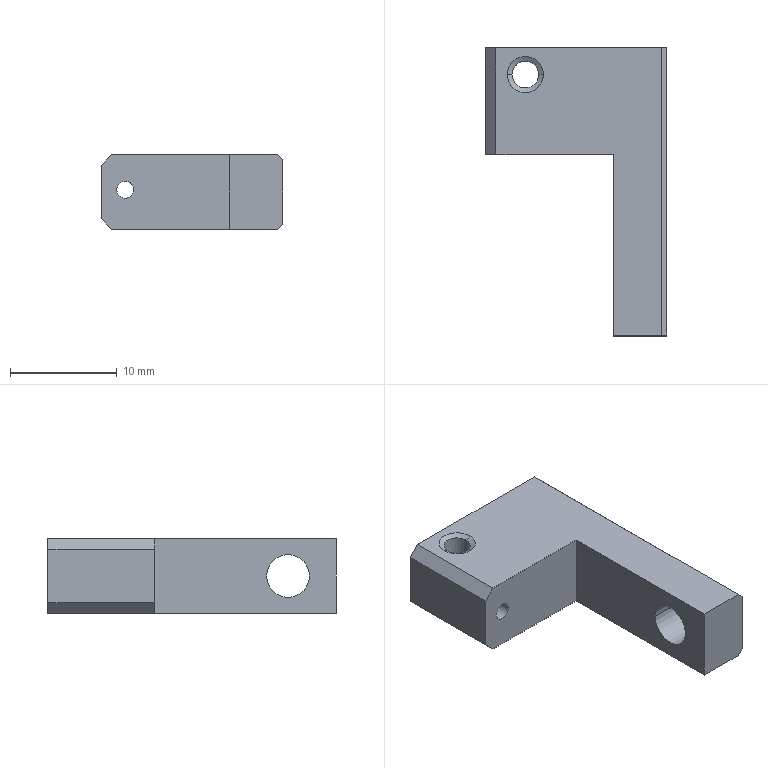Part | NX | 1 solid | 20 faces | box 17 x 27 x 7 mm | volume 1651 mm3 | plane 12 | cylinder 6 | cone 2 | commonest cylinder face diameters 1.6 x2 2.5 x2 4 x2
STEP:
#1=CARTESIAN_POINT('',(1.,17.,0.));
#2=VERTEX_POINT('',#1);
#3=CARTESIAN_POINT('',(12.,17.,0.));
#4=VERTEX_POINT('',#3);
#5=CARTESIAN_POINT('',(0.,17.,0.));
#6=DIRECTION('',(1.,0.,0.));
#7=VECTOR('',#6,1000.);
#8=LINE('',#5,#7);
#9=EDGE_CURVE('',#2,#4,#8,.T.);
#10=ORIENTED_EDGE('',*,*,#9,.T.);
#11=CARTESIAN_POINT('',(12.,17.,7.));
#12=VERTEX_POINT('',#11);
#13=CARTESIAN_POINT('',(12.,17.,0.));
#14=DIRECTION('',(0.,0.,1.));
#15=VECTOR('',#14,1000.);
#16=LINE('',#13,#15);
#17=EDGE_CURVE('',#4,#12,#16,.T.);
#18=ORIENTED_EDGE('',*,*,#17,.T.);
#19=CARTESIAN_POINT('',(1.,17.,7.));
#20=VERTEX_POINT('',#19);
#21=CARTESIAN_POINT('',(0.,17.,7.));
#22=DIRECTION('',(1.,0.,0.));
#23=VECTOR('',#22,1000.);
#24=LINE('',#21,#23);
#25=EDGE_CURVE('',#20,#12,#24,.T.);
#26=ORIENTED_EDGE('',*,*,#25,.F.);
#27=CARTESIAN_POINT('',(0.,17.,6.));
#28=VERTEX_POINT('',#27);
#29=CARTESIAN_POINT('',(-6.,17.,0.));
#30=DIRECTION('',(0.7071,0.,0.7071));
#31=VECTOR('',#30,1000.);
#32=LINE('',#29,#31);
#33=EDGE_CURVE('',#28,#20,#32,.T.);
#34=ORIENTED_EDGE('',*,*,#33,.F.);
#35=CARTESIAN_POINT('',(0.,17.,1.));
#36=VERTEX_POINT('',#35);
#37=CARTESIAN_POINT('',(0.,17.,0.));
#38=DIRECTION('',(0.,0.,-1.));
#39=VECTOR('',#38,1000.);
#40=LINE('',#37,#39);
#41=EDGE_CURVE('',#28,#36,#40,.T.);
#42=ORIENTED_EDGE('',*,*,#41,.T.);
#43=CARTESIAN_POINT('',(1.,17.,0.));
#44=DIRECTION('',(0.7071,0.,-0.7071));
#45=VECTOR('',#44,1000.);
#46=LINE('',#43,#45);
#47=EDGE_CURVE('',#36,#2,#46,.T.);
#48=ORIENTED_EDGE('',*,*,#47,.T.);
#49=EDGE_LOOP('',(#10,#18,#26,#34,#42,#48));
#50=FACE_BOUND('',#49,.T.);
#51=CARTESIAN_POINT('',(3.05,17.,3.7));
#52=VERTEX_POINT('',#51);
#53=CARTESIAN_POINT('',(1.45,17.,3.7));
#54=VERTEX_POINT('',#53);
#55=CARTESIAN_POINT('',(2.25,17.,3.7));
#56=DIRECTION('',(0.,-1.,0.));
#57=DIRECTION('',(1.,0.,0.));
#58=AXIS2_PLACEMENT_3D('',#55,#56,#57);
#59=CIRCLE('',#58,0.8);
#60=EDGE_CURVE('',#52,#54,#59,.T.);
#61=ORIENTED_EDGE('',*,*,#60,.F.);
#62=CARTESIAN_POINT('',(2.25,17.,3.7));
#63=DIRECTION('',(0.,-1.,0.));
#64=DIRECTION('',(1.,0.,0.));
#65=AXIS2_PLACEMENT_3D('',#62,#63,#64);
#66=CIRCLE('',#65,0.8);
#67=EDGE_CURVE('',#54,#52,#66,.T.);
#68=ORIENTED_EDGE('',*,*,#67,.F.);
#69=EDGE_LOOP('',(#61,#68));
#70=FACE_BOUND('',#69,.T.);
#71=CARTESIAN_POINT('',(12.,17.,7.));
#72=DIRECTION('',(0.,1.,0.));
#73=DIRECTION('',(1.,0.,0.));
#74=AXIS2_PLACEMENT_3D('',#71,#72,#73);
#75=PLANE('',#74);
#76=ADVANCED_FACE('',(#50,#70),#75,.F.);
#77=CARTESIAN_POINT('',(17.,27.,0.5));
#78=VERTEX_POINT('',#77);
#79=CARTESIAN_POINT('',(17.,0.,0.5));
#80=VERTEX_POINT('',#79);
#81=CARTESIAN_POINT('',(17.,27.,0.5));
#82=DIRECTION('',(0.,-1.,0.));
#83=VECTOR('',#82,1000.);
#84=LINE('',#81,#83);
#85=EDGE_CURVE('',#78,#80,#84,.T.);
#86=ORIENTED_EDGE('',*,*,#85,.F.);
#87=CARTESIAN_POINT('',(17.,27.,6.5));
#88=VERTEX_POINT('',#87);
#89=CARTESIAN_POINT('',(17.,27.,0.));
#90=DIRECTION('',(0.,0.,1.));
#91=VECTOR('',#90,1000.);
#92=LINE('',#89,#91);
#93=EDGE_CURVE('',#78,#88,#92,.T.);
#94=ORIENTED_EDGE('',*,*,#93,.T.);
#95=CARTESIAN_POINT('',(17.,0.,6.5));
#96=VERTEX_POINT('',#95);
#97=CARTESIAN_POINT('',(17.,27.,6.5));
#98=DIRECTION('',(0.,-1.,0.));
#99=VECTOR('',#98,1000.);
#100=LINE('',#97,#99);
#101=EDGE_CURVE('',#88,#96,#100,.T.);
#102=ORIENTED_EDGE('',*,*,#101,.T.);
#103=CARTESIAN_POINT('',(17.,0.,6.5));
#104=DIRECTION('',(0.,0.,-1.));
#105=VECTOR('',#104,1000.);
#106=LINE('',#103,#105);
#107=EDGE_CURVE('',#96,#80,#106,.T.);
#108=ORIENTED_EDGE('',*,*,#107,.T.);
#109=EDGE_LOOP('',(#86,#94,#102,#108));
#110=FACE_BOUND('',#109,.T.);
#111=CARTESIAN_POINT('',(17.,2.5,3.5));
#112=VERTEX_POINT('',#111);
#113=CARTESIAN_POINT('',(17.,6.5,3.5));
#114=VERTEX_POINT('',#113);
#115=CARTESIAN_POINT('',(17.,4.5,3.5));
#116=DIRECTION('',(1.,0.,0.));
#117=DIRECTION('',(0.,-1.,0.));
#118=AXIS2_PLACEMENT_3D('',#115,#116,#117);
#119=CIRCLE('',#118,2.);
#120=EDGE_CURVE('',#112,#114,#119,.T.);
#121=ORIENTED_EDGE('',*,*,#120,.F.);
#122=CARTESIAN_POINT('',(17.,4.5,3.5));
#123=DIRECTION('',(1.,0.,0.));
#124=DIRECTION('',(0.,-1.,0.));
#125=AXIS2_PLACEMENT_3D('',#122,#123,#124);
#126=CIRCLE('',#125,2.);
#127=EDGE_CURVE('',#114,#112,#126,.T.);
#128=ORIENTED_EDGE('',*,*,#127,.F.);
#129=EDGE_LOOP('',(#121,#128));
#130=FACE_BOUND('',#129,.T.);
#131=CARTESIAN_POINT('',(17.,0.,0.));
#132=DIRECTION('',(1.,0.,0.));
#133=DIRECTION('',(0.,1.,0.));
#134=AXIS2_PLACEMENT_3D('',#131,#132,#133);
#135=PLANE('',#134);
#136=ADVANCED_FACE('',(#110,#130),#135,.T.);
#137=CARTESIAN_POINT('',(12.,0.,7.));
#138=VERTEX_POINT('',#137);
#139=CARTESIAN_POINT('',(12.,0.,7.));
#140=DIRECTION('',(0.,-1.,0.));
#141=VECTOR('',#140,1000.);
#142=LINE('',#139,#141);
#143=EDGE_CURVE('',#12,#138,#142,.T.);
#144=ORIENTED_EDGE('',*,*,#143,.T.);
#145=CARTESIAN_POINT('',(16.5,0.,7.));
#146=VERTEX_POINT('',#145);
#147=CARTESIAN_POINT('',(0.,0.,7.));
#148=DIRECTION('',(-1.,0.,0.));
#149=VECTOR('',#148,1000.);
#150=LINE('',#147,#149);
#151=EDGE_CURVE('',#146,#138,#150,.T.);
#152=ORIENTED_EDGE('',*,*,#151,.F.);
#153=CARTESIAN_POINT('',(16.5,27.,7.));
#154=VERTEX_POINT('',#153);
#155=CARTESIAN_POINT('',(16.5,0.,7.));
#156=DIRECTION('',(0.,1.,0.));
#157=VECTOR('',#156,1000.);
#158=LINE('',#155,#157);
#159=EDGE_CURVE('',#146,#154,#158,.T.);
#160=ORIENTED_EDGE('',*,*,#159,.T.);
#161=CARTESIAN_POINT('',(1.,27.,7.));
#162=VERTEX_POINT('',#161);
#163=CARTESIAN_POINT('',(0.,27.,7.));
#164=DIRECTION('',(1.,0.,0.));
#165=VECTOR('',#164,1000.);
#166=LINE('',#163,#165);
#167=EDGE_CURVE('',#162,#154,#166,.T.);
#168=ORIENTED_EDGE('',*,*,#167,.F.);
#169=CARTESIAN_POINT('',(1.,0.,7.));
#170=DIRECTION('',(0.,-1.,0.));
#171=VECTOR('',#170,1000.);
#172=LINE('',#169,#171);
#173=EDGE_CURVE('',#162,#20,#172,.T.);
#174=ORIENTED_EDGE('',*,*,#173,.T.);
#175=ORIENTED_EDGE('',*,*,#25,.T.);
#176=EDGE_LOOP('',(#144,#152,#160,#168,#174,#175));
#177=FACE_BOUND('',#176,.T.);
#178=CARTESIAN_POINT('',(5.45,24.5,7.));
#179=VERTEX_POINT('',#178);
#180=CARTESIAN_POINT('',(2.05,24.5,7.));
#181=VERTEX_POINT('',#180);
#182=CARTESIAN_POINT('',(3.75,24.5,7.));
#183=DIRECTION('',(0.,0.,1.));
#184=DIRECTION('',(1.,0.,0.));
#185=AXIS2_PLACEMENT_3D('',#182,#183,#184);
#186=CIRCLE('',#185,1.7);
#187=EDGE_CURVE('',#179,#181,#186,.T.);
#188=ORIENTED_EDGE('',*,*,#187,.F.);
#189=CARTESIAN_POINT('',(3.75,24.5,7.));
#190=DIRECTION('',(0.,0.,1.));
#191=DIRECTION('',(1.,0.,0.));
#192=AXIS2_PLACEMENT_3D('',#189,#190,#191);
#193=CIRCLE('',#192,1.7);
#194=EDGE_CURVE('',#181,#179,#193,.T.);
#195=ORIENTED_EDGE('',*,*,#194,.F.);
#196=EDGE_LOOP('',(#188,#195));
#197=FACE_BOUND('',#196,.T.);
#198=CARTESIAN_POINT('',(0.,0.,7.));
#199=DIRECTION('',(0.,0.,1.));
#200=DIRECTION('',(1.,0.,0.));
#201=AXIS2_PLACEMENT_3D('',#198,#199,#200);
#202=PLANE('',#201);
#203=ADVANCED_FACE('',(#177,#197),#202,.T.);
#204=CARTESIAN_POINT('',(1.,27.,0.));
#205=VERTEX_POINT('',#204);
#206=CARTESIAN_POINT('',(1.,0.,0.));
#207=DIRECTION('',(0.,1.,0.));
#208=VECTOR('',#207,1000.);
#209=LINE('',#206,#208);
#210=EDGE_CURVE('',#2,#205,#209,.T.);
#211=ORIENTED_EDGE('',*,*,#210,.F.);
#212=ORIENTED_EDGE('',*,*,#47,.F.);
#213=CARTESIAN_POINT('',(0.,27.,1.));
#214=VERTEX_POINT('',#213);
#215=CARTESIAN_POINT('',(0.,17.,1.));
#216=DIRECTION('',(0.,1.,0.));
#217=VECTOR('',#216,1000.);
#218=LINE('',#215,#217);
#219=EDGE_CURVE('',#36,#214,#218,.T.);
#220=ORIENTED_EDGE('',*,*,#219,.T.);
#221=CARTESIAN_POINT('',(1.,27.,0.));
#222=DIRECTION('',(0.7071,0.,-0.7071));
#223=VECTOR('',#222,1000.);
#224=LINE('',#221,#223);
#225=EDGE_CURVE('',#214,#205,#224,.T.);
#226=ORIENTED_EDGE('',*,*,#225,.T.);
#227=EDGE_LOOP('',(#211,#212,#220,#226));
#228=FACE_BOUND('',#227,.T.);
#229=CARTESIAN_POINT('',(1.,27.,0.));
#230=DIRECTION('',(-0.7071,0.,-0.7071));
#231=DIRECTION('',(-0.7071,0.,0.7071));
#232=AXIS2_PLACEMENT_3D('',#229,#230,#231);
#233=PLANE('',#232);
#234=ADVANCED_FACE('',(#228),#233,.T.);
#235=CARTESIAN_POINT('',(12.,0.,0.));
#236=VERTEX_POINT('',#235);
#237=CARTESIAN_POINT('',(12.,0.,0.));
#238=DIRECTION('',(0.,-1.,0.));
#239=VECTOR('',#238,1000.);
#240=LINE('',#237,#239);
#241=EDGE_CURVE('',#4,#236,#240,.T.);
#242=ORIENTED_EDGE('',*,*,#241,.F.);
#243=ORIENTED_EDGE('',*,*,#9,.F.);
#244=ORIENTED_EDGE('',*,*,#210,.T.);
#245=CARTESIAN_POINT('',(16.5,27.,0.));
#246=VERTEX_POINT('',#245);
#247=CARTESIAN_POINT('',(0.,27.,0.));
#248=DIRECTION('',(1.,0.,0.));
#249=VECTOR('',#248,1000.);
#250=LINE('',#247,#249);
#251=EDGE_CURVE('',#205,#246,#250,.T.);
#252=ORIENTED_EDGE('',*,*,#251,.T.);
#253=CARTESIAN_POINT('',(16.5,0.,0.));
#254=VERTEX_POINT('',#253);
#255=CARTESIAN_POINT('',(16.5,0.,0.));
#256=DIRECTION('',(0.,-1.,0.));
#257=VECTOR('',#256,1000.);
#258=LINE('',#255,#257);
#259=EDGE_CURVE('',#246,#254,#258,.T.);
#260=ORIENTED_EDGE('',*,*,#259,.T.);
#261=CARTESIAN_POINT('',(0.,0.,0.));
#262=DIRECTION('',(-1.,0.,0.));
#263=VECTOR('',#262,1000.);
#264=LINE('',#261,#263);
#265=EDGE_CURVE('',#254,#236,#264,.T.);
#266=ORIENTED_EDGE('',*,*,#265,.T.);
#267=EDGE_LOOP('',(#242,#243,#244,#252,#260,#266));
#268=FACE_BOUND('',#267,.T.);
#269=CARTESIAN_POINT('',(5.,24.5,0.));
#270=VERTEX_POINT('',#269);
#271=CARTESIAN_POINT('',(2.5,24.5,0.));
#272=VERTEX_POINT('',#271);
#273=CARTESIAN_POINT('',(3.75,24.5,0.));
#274=DIRECTION('',(0.,0.,1.));
#275=DIRECTION('',(1.,0.,0.));
#276=AXIS2_PLACEMENT_3D('',#273,#274,#275);
#277=CIRCLE('',#276,1.25);
#278=EDGE_CURVE('',#270,#272,#277,.T.);
#279=ORIENTED_EDGE('',*,*,#278,.T.);
#280=CARTESIAN_POINT('',(3.75,24.5,0.));
#281=DIRECTION('',(0.,0.,1.));
#282=DIRECTION('',(1.,0.,0.));
#283=AXIS2_PLACEMENT_3D('',#280,#281,#282);
#284=CIRCLE('',#283,1.25);
#285=EDGE_CURVE('',#272,#270,#284,.T.);
#286=ORIENTED_EDGE('',*,*,#285,.T.);
#287=EDGE_LOOP('',(#279,#286));
#288=FACE_BOUND('',#287,.T.);
#289=CARTESIAN_POINT('',(0.,0.,0.));
#290=DIRECTION('',(0.,0.,1.));
#291=DIRECTION('',(1.,0.,0.));
#292=AXIS2_PLACEMENT_3D('',#289,#290,#291);
#293=PLANE('',#292);
#294=ADVANCED_FACE('',(#268,#288),#293,.F.);
#295=ORIENTED_EDGE('',*,*,#259,.F.);
#296=CARTESIAN_POINT('',(16.5,27.,0.));
#297=DIRECTION('',(0.7071,0.,0.7071));
#298=VECTOR('',#297,1000.);
#299=LINE('',#296,#298);
#300=EDGE_CURVE('',#246,#78,#299,.T.);
#301=ORIENTED_EDGE('',*,*,#300,.T.);
#302=ORIENTED_EDGE('',*,*,#85,.T.);
#303=CARTESIAN_POINT('',(17.,0.,0.5));
#304=DIRECTION('',(-0.7071,0.,-0.7071));
#305=VECTOR('',#304,1000.);
#306=LINE('',#303,#305);
#307=EDGE_CURVE('',#80,#254,#306,.T.);
#308=ORIENTED_EDGE('',*,*,#307,.T.);
#309=EDGE_LOOP('',(#295,#301,#302,#308));
#310=FACE_BOUND('',#309,.T.);
#311=CARTESIAN_POINT('',(16.5,0.,0.));
#312=DIRECTION('',(0.7071,0.,-0.7071));
#313=DIRECTION('',(0.,-1.,0.));
#314=AXIS2_PLACEMENT_3D('',#311,#312,#313);
#315=PLANE('',#314);
#316=ADVANCED_FACE('',(#310),#315,.T.);
#317=CARTESIAN_POINT('',(12.,0.,7.));
#318=DIRECTION('',(0.,0.,-1.));
#319=VECTOR('',#318,1000.);
#320=LINE('',#317,#319);
#321=EDGE_CURVE('',#138,#236,#320,.T.);
#322=ORIENTED_EDGE('',*,*,#321,.T.);
#323=ORIENTED_EDGE('',*,*,#265,.F.);
#324=ORIENTED_EDGE('',*,*,#307,.F.);
#325=ORIENTED_EDGE('',*,*,#107,.F.);
#326=CARTESIAN_POINT('',(16.5,0.,7.));
#327=DIRECTION('',(0.7071,0.,-0.7071));
#328=VECTOR('',#327,1000.);
#329=LINE('',#326,#328);
#330=EDGE_CURVE('',#146,#96,#329,.T.);
#331=ORIENTED_EDGE('',*,*,#330,.F.);
#332=ORIENTED_EDGE('',*,*,#151,.T.);
#333=EDGE_LOOP('',(#322,#323,#324,#325,#331,#332));
#334=FACE_BOUND('',#333,.T.);
#335=CARTESIAN_POINT('',(0.,0.,0.));
#336=DIRECTION('',(0.,-1.,0.));
#337=DIRECTION('',(0.,0.,-1.));
#338=AXIS2_PLACEMENT_3D('',#335,#336,#337);
#339=PLANE('',#338);
#340=ADVANCED_FACE('',(#334),#339,.T.);
#341=ORIENTED_EDGE('',*,*,#251,.F.);
#342=ORIENTED_EDGE('',*,*,#225,.F.);
#343=CARTESIAN_POINT('',(0.,27.,6.));
#344=VERTEX_POINT('',#343);
#345=CARTESIAN_POINT('',(0.,27.,0.));
#346=DIRECTION('',(0.,0.,-1.));
#347=VECTOR('',#346,1000.);
#348=LINE('',#345,#347);
#349=EDGE_CURVE('',#344,#214,#348,.T.);
#350=ORIENTED_EDGE('',*,*,#349,.F.);
#351=CARTESIAN_POINT('',(-6.,27.,0.));
#352=DIRECTION('',(0.7071,0.,0.7071));
#353=VECTOR('',#352,1000.);
#354=LINE('',#351,#353);
#355=EDGE_CURVE('',#344,#162,#354,.T.);
#356=ORIENTED_EDGE('',*,*,#355,.T.);
#357=ORIENTED_EDGE('',*,*,#167,.T.);
#358=CARTESIAN_POINT('',(23.5,27.,0.));
#359=DIRECTION('',(0.7071,0.,-0.7071));
#360=VECTOR('',#359,1000.);
#361=LINE('',#358,#360);
#362=EDGE_CURVE('',#154,#88,#361,.T.);
#363=ORIENTED_EDGE('',*,*,#362,.T.);
#364=ORIENTED_EDGE('',*,*,#93,.F.);
#365=ORIENTED_EDGE('',*,*,#300,.F.);
#366=EDGE_LOOP('',(#341,#342,#350,#356,#357,#363,#364,#365));
#367=FACE_BOUND('',#366,.T.);
#368=CARTESIAN_POINT('',(3.05,27.,3.7));
#369=VERTEX_POINT('',#368);
#370=CARTESIAN_POINT('',(1.45,27.,3.7));
#371=VERTEX_POINT('',#370);
#372=CARTESIAN_POINT('',(2.25,27.,3.7));
#373=DIRECTION('',(0.,-1.,0.));
#374=DIRECTION('',(1.,0.,0.));
#375=AXIS2_PLACEMENT_3D('',#372,#373,#374);
#376=CIRCLE('',#375,0.8);
#377=EDGE_CURVE('',#369,#371,#376,.T.);
#378=ORIENTED_EDGE('',*,*,#377,.T.);
#379=CARTESIAN_POINT('',(2.25,27.,3.7));
#380=DIRECTION('',(0.,-1.,0.));
#381=DIRECTION('',(1.,0.,0.));
#382=AXIS2_PLACEMENT_3D('',#379,#380,#381);
#383=CIRCLE('',#382,0.8);
#384=EDGE_CURVE('',#371,#369,#383,.T.);
#385=ORIENTED_EDGE('',*,*,#384,.T.);
#386=EDGE_LOOP('',(#378,#385));
#387=FACE_BOUND('',#386,.T.);
#388=CARTESIAN_POINT('',(17.,27.,0.));
#389=DIRECTION('',(0.,1.,0.));
#390=DIRECTION('',(1.,0.,0.));
#391=AXIS2_PLACEMENT_3D('',#388,#389,#390);
#392=PLANE('',#391);
#393=ADVANCED_FACE('',(#367,#387),#392,.T.);
#394=ORIENTED_EDGE('',*,*,#173,.F.);
#395=ORIENTED_EDGE('',*,*,#355,.F.);
#396=CARTESIAN_POINT('',(0.,17.,6.));
#397=DIRECTION('',(0.,1.,0.));
#398=VECTOR('',#397,1000.);
#399=LINE('',#396,#398);
#400=EDGE_CURVE('',#28,#344,#399,.T.);
#401=ORIENTED_EDGE('',*,*,#400,.F.);
#402=ORIENTED_EDGE('',*,*,#33,.T.);
#403=EDGE_LOOP('',(#394,#395,#401,#402));
#404=FACE_BOUND('',#403,.T.);
#405=CARTESIAN_POINT('',(1.,27.,7.));
#406=DIRECTION('',(0.7071,0.,-0.7071));
#407=DIRECTION('',(0.,-1.,0.));
#408=AXIS2_PLACEMENT_3D('',#405,#406,#407);
#409=PLANE('',#408);
#410=ADVANCED_FACE('',(#404),#409,.F.);
#411=ORIENTED_EDGE('',*,*,#41,.F.);
#412=ORIENTED_EDGE('',*,*,#400,.T.);
#413=ORIENTED_EDGE('',*,*,#349,.T.);
#414=ORIENTED_EDGE('',*,*,#219,.F.);
#415=EDGE_LOOP('',(#411,#412,#413,#414));
#416=FACE_BOUND('',#415,.T.);
#417=CARTESIAN_POINT('',(0.,27.,0.));
#418=DIRECTION('',(-1.,0.,0.));
#419=DIRECTION('',(0.,0.,1.));
#420=AXIS2_PLACEMENT_3D('',#417,#418,#419);
#421=PLANE('',#420);
#422=ADVANCED_FACE('',(#416),#421,.T.);
#423=ORIENTED_EDGE('',*,*,#159,.F.);
#424=ORIENTED_EDGE('',*,*,#330,.T.);
#425=ORIENTED_EDGE('',*,*,#101,.F.);
#426=ORIENTED_EDGE('',*,*,#362,.F.);
#427=EDGE_LOOP('',(#423,#424,#425,#426));
#428=FACE_BOUND('',#427,.T.);
#429=CARTESIAN_POINT('',(16.5,0.,7.));
#430=DIRECTION('',(-0.7071,0.,-0.7071));
#431=DIRECTION('',(-0.7071,0.,0.7071));
#432=AXIS2_PLACEMENT_3D('',#429,#430,#431);
#433=PLANE('',#432);
#434=ADVANCED_FACE('',(#428),#433,.F.);
#435=ORIENTED_EDGE('',*,*,#241,.T.);
#436=ORIENTED_EDGE('',*,*,#321,.F.);
#437=ORIENTED_EDGE('',*,*,#143,.F.);
#438=ORIENTED_EDGE('',*,*,#17,.F.);
#439=EDGE_LOOP('',(#435,#436,#437,#438));
#440=FACE_BOUND('',#439,.T.);
#441=CARTESIAN_POINT('',(12.,6.5,3.5));
#442=VERTEX_POINT('',#441);
#443=CARTESIAN_POINT('',(12.,2.5,3.5));
#444=VERTEX_POINT('',#443);
#445=CARTESIAN_POINT('',(12.,4.5,3.5));
#446=DIRECTION('',(-1.,0.,0.));
#447=DIRECTION('',(0.,1.,0.));
#448=AXIS2_PLACEMENT_3D('',#445,#446,#447);
#449=CIRCLE('',#448,2.);
#450=EDGE_CURVE('',#442,#444,#449,.T.);
#451=ORIENTED_EDGE('',*,*,#450,.F.);
#452=CARTESIAN_POINT('',(12.,4.5,3.5));
#453=DIRECTION('',(-1.,0.,0.));
#454=DIRECTION('',(0.,1.,0.));
#455=AXIS2_PLACEMENT_3D('',#452,#453,#454);
#456=CIRCLE('',#455,2.);
#457=EDGE_CURVE('',#444,#442,#456,.T.);
#458=ORIENTED_EDGE('',*,*,#457,.F.);
#459=EDGE_LOOP('',(#451,#458));
#460=FACE_BOUND('',#459,.T.);
#461=CARTESIAN_POINT('',(12.,0.,7.));
#462=DIRECTION('',(1.,0.,0.));
#463=DIRECTION('',(0.,1.,0.));
#464=AXIS2_PLACEMENT_3D('',#461,#462,#463);
#465=PLANE('',#464);
#466=ADVANCED_FACE('',(#440,#460),#465,.F.);
#467=ORIENTED_EDGE('',*,*,#450,.T.);
#468=CARTESIAN_POINT('',(17.,2.5,3.5));
#469=DIRECTION('',(-1.,0.,0.));
#470=VECTOR('',#469,1000.);
#471=LINE('',#468,#470);
#472=EDGE_CURVE('',#444,#112,#471,.F.);
#473=ORIENTED_EDGE('',*,*,#472,.T.);
#474=ORIENTED_EDGE('',*,*,#120,.T.);
#475=CARTESIAN_POINT('',(17.,6.5,3.5));
#476=DIRECTION('',(-1.,0.,0.));
#477=VECTOR('',#476,1000.);
#478=LINE('',#475,#477);
#479=EDGE_CURVE('',#442,#114,#478,.F.);
#480=ORIENTED_EDGE('',*,*,#479,.F.);
#481=EDGE_LOOP('',(#467,#473,#474,#480));
#482=FACE_BOUND('',#481,.T.);
#483=CARTESIAN_POINT('',(17.,4.5,3.5));
#484=DIRECTION('',(-1.,0.,0.));
#485=DIRECTION('',(0.,-1.,0.));
#486=AXIS2_PLACEMENT_3D('',#483,#484,#485);
#487=CYLINDRICAL_SURFACE('',#486,2.);
#488=ADVANCED_FACE('',(#482),#487,.F.);
#489=ORIENTED_EDGE('',*,*,#60,.T.);
#490=CARTESIAN_POINT('',(1.45,27.,3.7));
#491=DIRECTION('',(0.,-1.,0.));
#492=VECTOR('',#491,1000.);
#493=LINE('',#490,#492);
#494=EDGE_CURVE('',#54,#371,#493,.F.);
#495=ORIENTED_EDGE('',*,*,#494,.T.);
#496=ORIENTED_EDGE('',*,*,#377,.F.);
#497=CARTESIAN_POINT('',(3.05,25.536,3.7));
#498=VERTEX_POINT('',#497);
#499=CARTESIAN_POINT('',(3.05,27.,3.7));
#500=DIRECTION('',(0.,-1.,0.));
#501=VECTOR('',#500,1000.);
#502=LINE('',#499,#501);
#503=EDGE_CURVE('',#369,#498,#502,.T.);
#504=ORIENTED_EDGE('',*,*,#503,.T.);
#505=CARTESIAN_POINT('',(2.5,24.5,4.46));
#506=VERTEX_POINT('',#505);
#507=CARTESIAN_POINT('',(3.05,25.536,3.7));
#508=CARTESIAN_POINT('',(3.05,25.536,3.983));
#509=CARTESIAN_POINT('',(2.709,25.323,4.44));
#510=CARTESIAN_POINT('',(2.5,24.776,4.46));
#511=CARTESIAN_POINT('',(2.5,24.5,4.46));
#512=B_SPLINE_CURVE_WITH_KNOTS('',3,(#507,#508,#509,#510,#511),.UNSPECIFIED.,.F.,.F.,(4,1,4),(0.,0.5,1.),.UNSPECIFIED.);
#513=EDGE_CURVE('',#498,#506,#512,.T.);
#514=ORIENTED_EDGE('',*,*,#513,.T.);
#515=CARTESIAN_POINT('',(3.05,23.464,3.7));
#516=VERTEX_POINT('',#515);
#517=CARTESIAN_POINT('',(2.5,24.5,4.46));
#518=CARTESIAN_POINT('',(2.5,24.224,4.46));
#519=CARTESIAN_POINT('',(2.709,23.677,4.44));
#520=CARTESIAN_POINT('',(3.05,23.464,3.983));
#521=CARTESIAN_POINT('',(3.05,23.464,3.7));
#522=B_SPLINE_CURVE_WITH_KNOTS('',3,(#517,#518,#519,#520,#521),.UNSPECIFIED.,.F.,.F.,(4,1,4),(0.,0.5,1.),.UNSPECIFIED.);
#523=EDGE_CURVE('',#506,#516,#522,.T.);
#524=ORIENTED_EDGE('',*,*,#523,.T.);
#525=CARTESIAN_POINT('',(3.05,27.,3.7));
#526=DIRECTION('',(0.,-1.,0.));
#527=VECTOR('',#526,1000.);
#528=LINE('',#525,#527);
#529=EDGE_CURVE('',#52,#516,#528,.F.);
#530=ORIENTED_EDGE('',*,*,#529,.F.);
#531=EDGE_LOOP('',(#489,#495,#496,#504,#514,#524,#530));
#532=FACE_BOUND('',#531,.T.);
#533=CARTESIAN_POINT('',(2.25,27.,3.7));
#534=DIRECTION('',(0.,-1.,0.));
#535=DIRECTION('',(1.,0.,0.));
#536=AXIS2_PLACEMENT_3D('',#533,#534,#535);
#537=CYLINDRICAL_SURFACE('',#536,0.8);
#538=ADVANCED_FACE('',(#532),#537,.F.);
#539=CARTESIAN_POINT('',(5.,24.5,6.74));
#540=VERTEX_POINT('',#539);
#541=CARTESIAN_POINT('',(2.5,24.5,6.74));
#542=VERTEX_POINT('',#541);
#543=CARTESIAN_POINT('',(3.75,24.5,6.74));
#544=DIRECTION('',(0.,0.,1.));
#545=DIRECTION('',(1.,0.,0.));
#546=AXIS2_PLACEMENT_3D('',#543,#544,#545);
#547=CIRCLE('',#546,1.25);
#548=EDGE_CURVE('',#540,#542,#547,.T.);
#549=ORIENTED_EDGE('',*,*,#548,.T.);
#550=CARTESIAN_POINT('',(2.5,24.5,7.));
#551=DIRECTION('',(0.,0.,1.));
#552=VECTOR('',#551,1000.);
#553=LINE('',#550,#552);
#554=EDGE_CURVE('',#542,#506,#553,.F.);
#555=ORIENTED_EDGE('',*,*,#554,.T.);
#556=ORIENTED_EDGE('',*,*,#513,.F.);
#557=CARTESIAN_POINT('',(2.5,24.5,2.94));
#558=VERTEX_POINT('',#557);
#559=CARTESIAN_POINT('',(3.05,25.536,3.7));
#560=CARTESIAN_POINT('',(3.05,25.536,3.422));
#561=CARTESIAN_POINT('',(2.709,25.315,2.958));
#562=CARTESIAN_POINT('',(2.5,24.793,2.94));
#563=CARTESIAN_POINT('',(2.5,24.5,2.94));
#564=B_SPLINE_CURVE_WITH_KNOTS('',3,(#559,#560,#561,#562,#563),.UNSPECIFIED.,.F.,.F.,(4,1,4),(0.,0.5,1.),.UNSPECIFIED.);
#565=EDGE_CURVE('',#558,#498,#564,.F.);
#566=ORIENTED_EDGE('',*,*,#565,.F.);
#567=CARTESIAN_POINT('',(2.5,24.5,7.));
#568=DIRECTION('',(0.,0.,1.));
#569=VECTOR('',#568,1000.);
#570=LINE('',#567,#569);
#571=EDGE_CURVE('',#272,#558,#570,.T.);
#572=ORIENTED_EDGE('',*,*,#571,.F.);
#573=ORIENTED_EDGE('',*,*,#278,.F.);
#574=CARTESIAN_POINT('',(5.,24.5,7.));
#575=DIRECTION('',(0.,0.,1.));
#576=VECTOR('',#575,1000.);
#577=LINE('',#574,#576);
#578=EDGE_CURVE('',#540,#270,#577,.F.);
#579=ORIENTED_EDGE('',*,*,#578,.F.);
#580=EDGE_LOOP('',(#549,#555,#556,#566,#572,#573,#579));
#581=FACE_BOUND('',#580,.T.);
#582=CARTESIAN_POINT('',(3.75,24.5,7.));
#583=DIRECTION('',(0.,0.,1.));
#584=DIRECTION('',(1.,0.,0.));
#585=AXIS2_PLACEMENT_3D('',#582,#583,#584);
#586=CYLINDRICAL_SURFACE('',#585,1.25);
#587=ADVANCED_FACE('',(#581),#586,.F.);
#588=ORIENTED_EDGE('',*,*,#548,.F.);
#589=CARTESIAN_POINT('',(5.,24.5,6.74));
#590=DIRECTION('',(0.866,0.,0.5));
#591=VECTOR('',#590,1000.);
#592=LINE('',#589,#591);
#593=EDGE_CURVE('',#540,#179,#592,.T.);
#594=ORIENTED_EDGE('',*,*,#593,.T.);
#595=ORIENTED_EDGE('',*,*,#187,.T.);
#596=CARTESIAN_POINT('',(2.5,24.5,6.74));
#597=DIRECTION('',(-0.866,0.,0.5));
#598=VECTOR('',#597,1000.);
#599=LINE('',#596,#598);
#600=EDGE_CURVE('',#542,#181,#599,.T.);
#601=ORIENTED_EDGE('',*,*,#600,.F.);
#602=EDGE_LOOP('',(#588,#594,#595,#601));
#603=FACE_BOUND('',#602,.T.);
#604=CARTESIAN_POINT('',(3.75,24.5,6.74));
#605=DIRECTION('',(0.,0.,1.));
#606=DIRECTION('',(1.,0.,0.));
#607=AXIS2_PLACEMENT_3D('',#604,#605,#606);
#608=CONICAL_SURFACE('',#607,1.25,1.047);
#609=ADVANCED_FACE('',(#603),#608,.F.);
#610=ORIENTED_EDGE('',*,*,#593,.F.);
#611=CARTESIAN_POINT('',(3.75,24.5,6.74));
#612=DIRECTION('',(0.,0.,1.));
#613=DIRECTION('',(1.,0.,0.));
#614=AXIS2_PLACEMENT_3D('',#611,#612,#613);
#615=CIRCLE('',#614,1.25);
#616=EDGE_CURVE('',#542,#540,#615,.T.);
#617=ORIENTED_EDGE('',*,*,#616,.F.);
#618=ORIENTED_EDGE('',*,*,#600,.T.);
#619=ORIENTED_EDGE('',*,*,#194,.T.);
#620=EDGE_LOOP('',(#610,#617,#618,#619));
#621=FACE_BOUND('',#620,.T.);
#622=CARTESIAN_POINT('',(3.75,24.5,6.74));
#623=DIRECTION('',(0.,0.,1.));
#624=DIRECTION('',(1.,0.,0.));
#625=AXIS2_PLACEMENT_3D('',#622,#623,#624);
#626=CONICAL_SURFACE('',#625,1.25,1.047);
#627=ADVANCED_FACE('',(#621),#626,.F.);
#628=CARTESIAN_POINT('',(2.5,24.5,2.94));
#629=CARTESIAN_POINT('',(2.5,24.204,2.94));
#630=CARTESIAN_POINT('',(2.709,23.687,2.958));
#631=CARTESIAN_POINT('',(3.05,23.464,3.421));
#632=CARTESIAN_POINT('',(3.05,23.464,3.7));
#633=B_SPLINE_CURVE_WITH_KNOTS('',3,(#628,#629,#630,#631,#632),.UNSPECIFIED.,.F.,.F.,(4,1,4),(0.,0.5,1.),.UNSPECIFIED.);
#634=EDGE_CURVE('',#516,#558,#633,.F.);
#635=ORIENTED_EDGE('',*,*,#634,.F.);
#636=ORIENTED_EDGE('',*,*,#523,.F.);
#637=ORIENTED_EDGE('',*,*,#554,.F.);
#638=ORIENTED_EDGE('',*,*,#616,.T.);
#639=ORIENTED_EDGE('',*,*,#578,.T.);
#640=ORIENTED_EDGE('',*,*,#285,.F.);
#641=ORIENTED_EDGE('',*,*,#571,.T.);
#642=EDGE_LOOP('',(#635,#636,#637,#638,#639,#640,#641));
#643=FACE_BOUND('',#642,.T.);
#644=CARTESIAN_POINT('',(3.75,24.5,7.));
#645=DIRECTION('',(0.,0.,1.));
#646=DIRECTION('',(1.,0.,0.));
#647=AXIS2_PLACEMENT_3D('',#644,#645,#646);
#648=CYLINDRICAL_SURFACE('',#647,1.25);
#649=ADVANCED_FACE('',(#643),#648,.F.);
#650=ORIENTED_EDGE('',*,*,#472,.F.);
#651=ORIENTED_EDGE('',*,*,#457,.T.);
#652=ORIENTED_EDGE('',*,*,#479,.T.);
#653=ORIENTED_EDGE('',*,*,#127,.T.);
#654=EDGE_LOOP('',(#650,#651,#652,#653));
#655=FACE_BOUND('',#654,.T.);
#656=CARTESIAN_POINT('',(17.,4.5,3.5));
#657=DIRECTION('',(-1.,0.,0.));
#658=DIRECTION('',(0.,-1.,0.));
#659=AXIS2_PLACEMENT_3D('',#656,#657,#658);
#660=CYLINDRICAL_SURFACE('',#659,2.);
#661=ADVANCED_FACE('',(#655),#660,.F.);
#662=ORIENTED_EDGE('',*,*,#634,.T.);
#663=ORIENTED_EDGE('',*,*,#565,.T.);
#664=ORIENTED_EDGE('',*,*,#503,.F.);
#665=ORIENTED_EDGE('',*,*,#384,.F.);
#666=ORIENTED_EDGE('',*,*,#494,.F.);
#667=ORIENTED_EDGE('',*,*,#67,.T.);
#668=ORIENTED_EDGE('',*,*,#529,.T.);
#669=EDGE_LOOP('',(#662,#663,#664,#665,#666,#667,#668));
#670=FACE_BOUND('',#669,.T.);
#671=CARTESIAN_POINT('',(2.25,27.,3.7));
#672=DIRECTION('',(0.,-1.,0.));
#673=DIRECTION('',(1.,0.,0.));
#674=AXIS2_PLACEMENT_3D('',#671,#672,#673);
#675=CYLINDRICAL_SURFACE('',#674,0.8);
#676=ADVANCED_FACE('',(#670),#675,.F.);
#677=CLOSED_SHELL('',(#76,#136,#203,#234,#294,#316,#340,#393,#410,#422,#434,#466,#488,#538,#587,#609,#627,#649,#661,#676));
#678=MANIFOLD_SOLID_BREP('',#677);
#679=(LENGTH_UNIT()NAMED_UNIT(*)SI_UNIT(.MILLI.,.METRE.));
#680=UNCERTAINTY_MEASURE_WITH_UNIT(LENGTH_MEASURE(0.0508),#679,'','');
#681=(NAMED_UNIT(*)PLANE_ANGLE_UNIT()SI_UNIT($,.RADIAN.));
#682=(NAMED_UNIT(*)SI_UNIT($,.STERADIAN.)SOLID_ANGLE_UNIT());
#683=(GEOMETRIC_REPRESENTATION_CONTEXT(3)GLOBAL_UNCERTAINTY_ASSIGNED_CONTEXT((#680))GLOBAL_UNIT_ASSIGNED_CONTEXT((#679,#681,#682))REPRESENTATION_CONTEXT('',''));
#684=ADVANCED_BREP_SHAPE_REPRESENTATION('',(#678),#683);